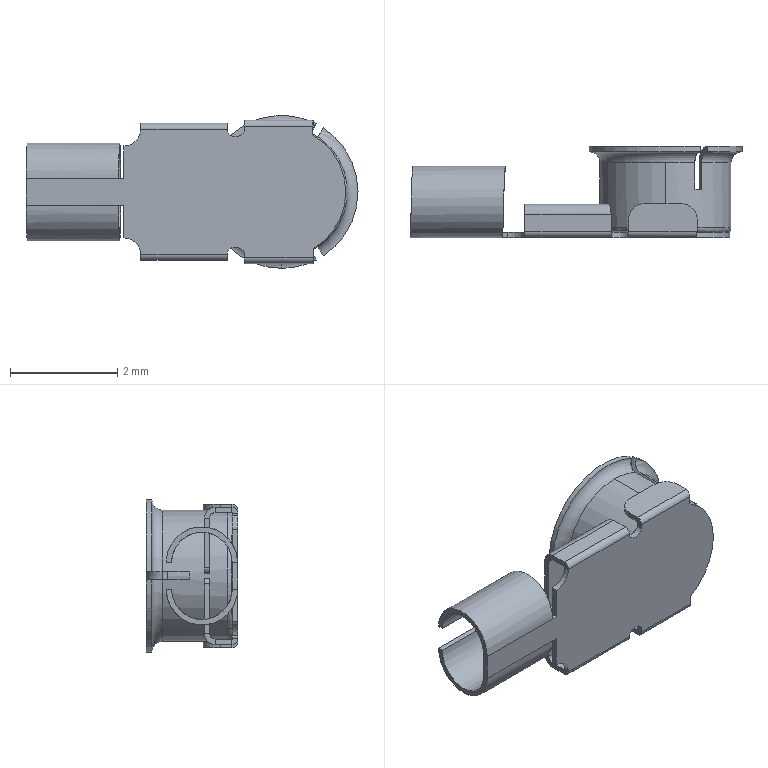Part | SolidWorks | features ICE 5, EdgeFlange 3, FlatPattern 1, Hem 1, MirrorPattern 1, Revolution 1, SMBaseFlange 1, SheetMetal 1 | 1 solid | 147 faces | box 6.189 x 1.7 x 2.85 mm | volume 6.846 mm3 | plane 84 | cylinder 47 | torus 10 | spline 6 | commonest cylinder face diameters 0.2 x6 0.02 x4 0.22 x4 0.64 x4 2.25 x4 2.85 x4